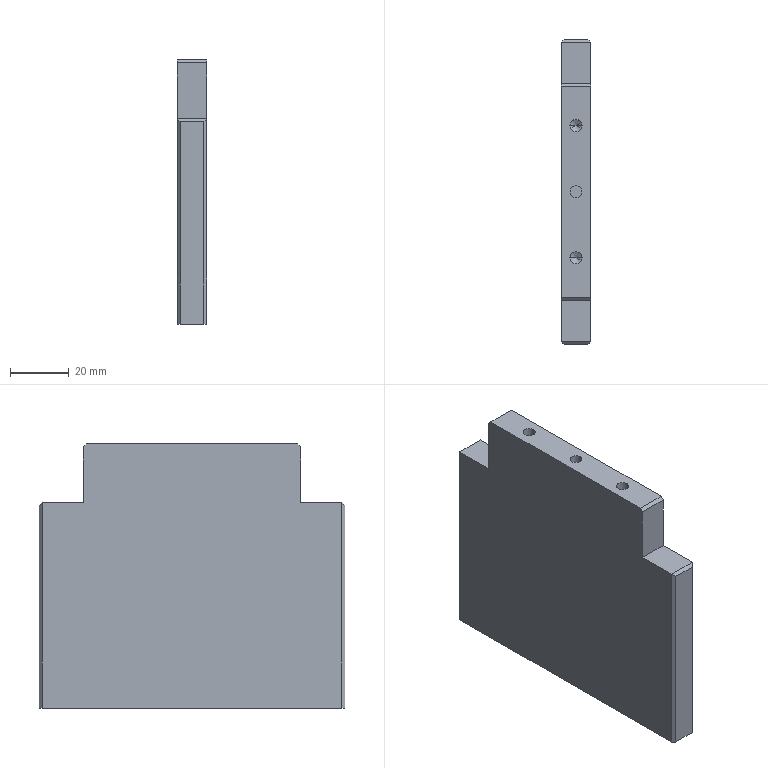Part | STEP file | CON-011 | 1 solid | 40 faces | box 10 x 104 x 90 mm | volume 86051 mm3 | plane 20 | cylinder 12 | cone 8 | commonest cylinder face diameters 4.2 x8 4 x4